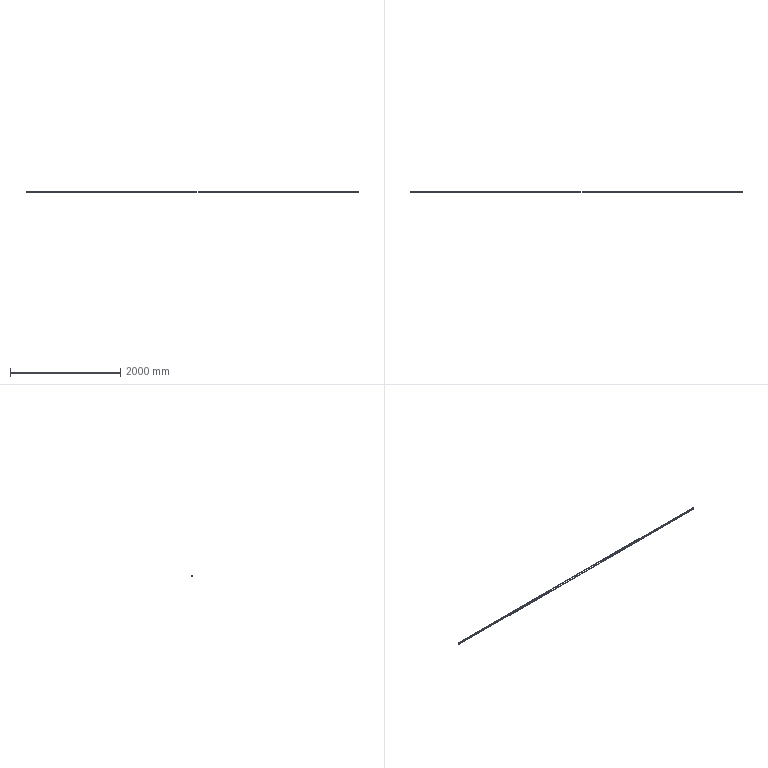Part | STEP file | ASND-0110-Q2 | 1 solid | 12 faces | box 6033 x 32.8 x 10 mm | volume 266115 mm3 | cylinder 6 | plane 6 | commonest cylinder face diameters 28.4 x3 32.8 x3
STEP:
#1=CARTESIAN_POINT('',(0.,0.,0.));
#2=DIRECTION('',(0.,0.,1.));
#3=DIRECTION('',(1.,0.,0.));
#4=AXIS2_PLACEMENT_3D('',#1,#2,#3);
#5=CARTESIAN_POINT('',(6000.,14.2,-140.));
#6=VERTEX_POINT('',#5);
#7=CARTESIAN_POINT('',(6000.,14.2,-130.));
#8=VERTEX_POINT('',#7);
#9=CARTESIAN_POINT('',(6000.,14.2,-140.));
#10=DIRECTION('',(0.,0.,1.));
#11=VECTOR('',#10,1.);
#12=LINE('',#9,#11);
#13=CARTESIAN_POINT('',(6000.,0.,-130.));
#14=DIRECTION('',(0.,0.,1.));
#15=DIRECTION('',(1.,0.,0.));
#16=AXIS2_PLACEMENT_3D('',#13,#14,#15);
#17=CYLINDRICAL_SURFACE('',#16,14.2);
#18=CARTESIAN_POINT('',(1.571,-10.));
#19=DIRECTION('',(0.,1.));
#20=VECTOR('',#19,1.);
#21=LINE('',#18,#20);
#22=(GEOMETRIC_REPRESENTATION_CONTEXT(2)PARAMETRIC_REPRESENTATION_CONTEXT()REPRESENTATION_CONTEXT('',''));
#23=DEFINITIONAL_REPRESENTATION('',(#21),#22);
#24=PCURVE('',#17,#23);
#25=CARTESIAN_POINT('',(0.,14.2,-130.));
#26=DIRECTION('',(0.,-1.,0.));
#27=DIRECTION('',(0.7071,0.,0.7071));
#28=AXIS2_PLACEMENT_3D('',#25,#26,#27);
#29=PLANE('',#28);
#30=CARTESIAN_POINT('',(4235.57,-4249.712));
#31=DIRECTION('',(0.7071,0.7071));
#32=VECTOR('',#31,1.);
#33=LINE('',#30,#32);
#34=(GEOMETRIC_REPRESENTATION_CONTEXT(2)PARAMETRIC_REPRESENTATION_CONTEXT()REPRESENTATION_CONTEXT('',''));
#35=DEFINITIONAL_REPRESENTATION('',(#33),#34);
#36=PCURVE('',#29,#35);
#37=SURFACE_CURVE('',#12,(#24,#36),.PCURVE_S1.);
#38=EDGE_CURVE('',#6,#8,#37,.T.);
#39=ORIENTED_EDGE('',*,*,#38,.T.);
#40=CARTESIAN_POINT('',(6014.2,0.,-130.));
#41=VERTEX_POINT('',#40);
#42=CARTESIAN_POINT('',(6000.,0.,-130.));
#43=DIRECTION('',(0.,0.,-1.));
#44=DIRECTION('',(1.,0.,0.));
#45=AXIS2_PLACEMENT_3D('',#42,#43,#44);
#46=CIRCLE('',#45,14.2);
#47=CARTESIAN_POINT('',(6.283,0.));
#48=DIRECTION('',(-1.,0.));
#49=VECTOR('',#48,1.);
#50=LINE('',#47,#49);
#51=(GEOMETRIC_REPRESENTATION_CONTEXT(2)PARAMETRIC_REPRESENTATION_CONTEXT()REPRESENTATION_CONTEXT('',''));
#52=DEFINITIONAL_REPRESENTATION('',(#50),#51);
#53=PCURVE('',#17,#52);
#54=CARTESIAN_POINT('',(0.,0.,-130.));
#55=DIRECTION('',(0.,0.,1.));
#56=DIRECTION('',(0.7071,0.7071,0.));
#57=AXIS2_PLACEMENT_3D('',#54,#55,#56);
#58=PLANE('',#57);
#59=CARTESIAN_POINT('',(4252.682,-4252.682));
#60=CARTESIAN_POINT('',(4235.29,-4270.073));
#61=CARTESIAN_POINT('',(4228.925,-4246.316));
#62=CARTESIAN_POINT('',(4222.559,-4222.559));
#63=CARTESIAN_POINT('',(4246.316,-4228.925));
#64=CARTESIAN_POINT('',(4270.073,-4235.29));
#65=CARTESIAN_POINT('',(4252.682,-4252.682));
#66=(BOUNDED_CURVE()B_SPLINE_CURVE(2,(#59,#60,#61,#62,#63,#64,#65),.UNSPECIFIED.,.T.,.F.)B_SPLINE_CURVE_WITH_KNOTS((1,2,2,2,2,1),(-2.094,0.,2.094,4.189,6.283,8.378),.UNSPECIFIED.)CURVE()GEOMETRIC_REPRESENTATION_ITEM()RATIONAL_B_SPLINE_CURVE((1.,0.5,1.,0.5,1.,0.5,1.))REPRESENTATION_ITEM(''));
#67=(GEOMETRIC_REPRESENTATION_CONTEXT(2)PARAMETRIC_REPRESENTATION_CONTEXT()REPRESENTATION_CONTEXT('',''));
#68=DEFINITIONAL_REPRESENTATION('',(#66),#67);
#69=PCURVE('',#58,#68);
#70=SURFACE_CURVE('',#46,(#53,#69),.PCURVE_S1.);
#71=EDGE_CURVE('',#8,#41,#70,.T.);
#72=ORIENTED_EDGE('',*,*,#71,.T.);
#73=CARTESIAN_POINT('',(6014.2,0.,-140.));
#74=VERTEX_POINT('',#73);
#75=CARTESIAN_POINT('',(6014.2,0.,-130.));
#76=DIRECTION('',(0.,0.,1.));
#77=VECTOR('',#76,1.);
#78=LINE('',#75,#77);
#79=CARTESIAN_POINT('',(0.,0.));
#80=DIRECTION('',(0.,1.));
#81=VECTOR('',#80,1.);
#82=LINE('',#79,#81);
#83=(GEOMETRIC_REPRESENTATION_CONTEXT(2)PARAMETRIC_REPRESENTATION_CONTEXT()REPRESENTATION_CONTEXT('',''));
#84=DEFINITIONAL_REPRESENTATION('',(#82),#83);
#85=PCURVE('',#17,#84);
#86=CARTESIAN_POINT('',(6000.,0.,-130.));
#87=DIRECTION('',(0.,0.,1.));
#88=DIRECTION('',(1.,0.,0.));
#89=AXIS2_PLACEMENT_3D('',#86,#87,#88);
#90=CYLINDRICAL_SURFACE('',#89,14.2);
#91=CARTESIAN_POINT('',(6.283,0.));
#92=DIRECTION('',(0.,1.));
#93=VECTOR('',#92,1.);
#94=LINE('',#91,#93);
#95=(GEOMETRIC_REPRESENTATION_CONTEXT(2)PARAMETRIC_REPRESENTATION_CONTEXT()REPRESENTATION_CONTEXT('',''));
#96=DEFINITIONAL_REPRESENTATION('',(#94),#95);
#97=PCURVE('',#90,#96);
#98=SURFACE_CURVE('',#78,(#85,#97),.PCURVE_S1.);
#99=EDGE_CURVE('',#74,#41,#98,.T.);
#100=ORIENTED_EDGE('',*,*,#99,.F.);
#101=CARTESIAN_POINT('',(6000.,0.,-140.));
#102=DIRECTION('',(0.,0.,1.));
#103=DIRECTION('',(1.,0.,0.));
#104=AXIS2_PLACEMENT_3D('',#101,#102,#103);
#105=CIRCLE('',#104,14.2);
#106=CARTESIAN_POINT('',(0.,-10.));
#107=DIRECTION('',(1.,0.));
#108=VECTOR('',#107,1.);
#109=LINE('',#106,#108);
#110=(GEOMETRIC_REPRESENTATION_CONTEXT(2)PARAMETRIC_REPRESENTATION_CONTEXT()REPRESENTATION_CONTEXT('',''));
#111=DEFINITIONAL_REPRESENTATION('',(#109),#110);
#112=PCURVE('',#17,#111);
#113=CARTESIAN_POINT('',(0.,0.,-140.));
#114=DIRECTION('',(0.,0.,1.));
#115=DIRECTION('',(0.7071,0.7071,0.));
#116=AXIS2_PLACEMENT_3D('',#113,#114,#115);
#117=PLANE('',#116);
#118=CARTESIAN_POINT('',(4242.641,-4242.641));
#119=DIRECTION('',(0.7071,-0.7071));
#120=AXIS2_PLACEMENT_2D('',#118,#119);
#121=CIRCLE('',#120,14.2);
#122=(GEOMETRIC_REPRESENTATION_CONTEXT(2)PARAMETRIC_REPRESENTATION_CONTEXT()REPRESENTATION_CONTEXT('',''));
#123=DEFINITIONAL_REPRESENTATION('',(#121),#122);
#124=PCURVE('',#117,#123);
#125=SURFACE_CURVE('',#105,(#112,#124),.PCURVE_S1.);
#126=EDGE_CURVE('',#74,#6,#125,.T.);
#127=ORIENTED_EDGE('',*,*,#126,.T.);
#128=EDGE_LOOP('',(#39,#72,#100,#127));
#129=FACE_BOUND('',#128,.F.);
#130=ADVANCED_FACE('',(#129),#17,.F.);
#131=CARTESIAN_POINT('',(6000.,-16.4,-140.));
#132=VERTEX_POINT('',#131);
#133=CARTESIAN_POINT('',(6016.4,0.,-140.));
#134=VERTEX_POINT('',#133);
#135=CARTESIAN_POINT('',(6000.,0.,-140.));
#136=DIRECTION('',(0.,0.,1.));
#137=DIRECTION('',(1.,0.,0.));
#138=AXIS2_PLACEMENT_3D('',#135,#136,#137);
#139=CIRCLE('',#138,16.4);
#140=CARTESIAN_POINT('',(6000.,0.,-130.));
#141=DIRECTION('',(0.,0.,1.));
#142=DIRECTION('',(1.,0.,0.));
#143=AXIS2_PLACEMENT_3D('',#140,#141,#142);
#144=CYLINDRICAL_SURFACE('',#143,16.4);
#145=CARTESIAN_POINT('',(0.,-10.));
#146=DIRECTION('',(1.,0.));
#147=VECTOR('',#146,1.);
#148=LINE('',#145,#147);
#149=(GEOMETRIC_REPRESENTATION_CONTEXT(2)PARAMETRIC_REPRESENTATION_CONTEXT()REPRESENTATION_CONTEXT('',''));
#150=DEFINITIONAL_REPRESENTATION('',(#148),#149);
#151=PCURVE('',#144,#150);
#152=CARTESIAN_POINT('',(4242.641,-4242.641));
#153=DIRECTION('',(0.7071,-0.7071));
#154=AXIS2_PLACEMENT_2D('',#152,#153);
#155=CIRCLE('',#154,16.4);
#156=(GEOMETRIC_REPRESENTATION_CONTEXT(2)PARAMETRIC_REPRESENTATION_CONTEXT()REPRESENTATION_CONTEXT('',''));
#157=DEFINITIONAL_REPRESENTATION('',(#155),#156);
#158=PCURVE('',#117,#157);
#159=SURFACE_CURVE('',#139,(#151,#158),.PCURVE_S1.);
#160=EDGE_CURVE('',#132,#134,#159,.T.);
#161=ORIENTED_EDGE('',*,*,#160,.T.);
#162=CARTESIAN_POINT('',(6016.4,0.,-130.));
#163=VERTEX_POINT('',#162);
#164=CARTESIAN_POINT('',(6016.4,0.,-130.));
#165=DIRECTION('',(0.,0.,1.));
#166=VECTOR('',#165,1.);
#167=LINE('',#164,#166);
#168=CARTESIAN_POINT('',(6.283,0.));
#169=DIRECTION('',(0.,1.));
#170=VECTOR('',#169,1.);
#171=LINE('',#168,#170);
#172=(GEOMETRIC_REPRESENTATION_CONTEXT(2)PARAMETRIC_REPRESENTATION_CONTEXT()REPRESENTATION_CONTEXT('',''));
#173=DEFINITIONAL_REPRESENTATION('',(#171),#172);
#174=PCURVE('',#144,#173);
#175=CARTESIAN_POINT('',(6000.,0.,-130.));
#176=DIRECTION('',(0.,0.,1.));
#177=DIRECTION('',(1.,0.,0.));
#178=AXIS2_PLACEMENT_3D('',#175,#176,#177);
#179=CYLINDRICAL_SURFACE('',#178,16.4);
#180=CARTESIAN_POINT('',(0.,0.));
#181=DIRECTION('',(0.,1.));
#182=VECTOR('',#181,1.);
#183=LINE('',#180,#182);
#184=(GEOMETRIC_REPRESENTATION_CONTEXT(2)PARAMETRIC_REPRESENTATION_CONTEXT()REPRESENTATION_CONTEXT('',''));
#185=DEFINITIONAL_REPRESENTATION('',(#183),#184);
#186=PCURVE('',#179,#185);
#187=SURFACE_CURVE('',#167,(#174,#186),.PCURVE_S1.);
#188=EDGE_CURVE('',#134,#163,#187,.T.);
#189=ORIENTED_EDGE('',*,*,#188,.T.);
#190=CARTESIAN_POINT('',(6000.,-16.4,-130.));
#191=VERTEX_POINT('',#190);
#192=CARTESIAN_POINT('',(6000.,0.,-130.));
#193=DIRECTION('',(0.,0.,1.));
#194=DIRECTION('',(1.,0.,0.));
#195=AXIS2_PLACEMENT_3D('',#192,#193,#194);
#196=CIRCLE('',#195,16.4);
#197=CARTESIAN_POINT('',(0.,0.));
#198=DIRECTION('',(1.,0.));
#199=VECTOR('',#198,1.);
#200=LINE('',#197,#199);
#201=(GEOMETRIC_REPRESENTATION_CONTEXT(2)PARAMETRIC_REPRESENTATION_CONTEXT()REPRESENTATION_CONTEXT('',''));
#202=DEFINITIONAL_REPRESENTATION('',(#200),#201);
#203=PCURVE('',#144,#202);
#204=CARTESIAN_POINT('',(4242.641,-4242.641));
#205=DIRECTION('',(0.7071,-0.7071));
#206=AXIS2_PLACEMENT_2D('',#204,#205);
#207=CIRCLE('',#206,16.4);
#208=(GEOMETRIC_REPRESENTATION_CONTEXT(2)PARAMETRIC_REPRESENTATION_CONTEXT()REPRESENTATION_CONTEXT('',''));
#209=DEFINITIONAL_REPRESENTATION('',(#207),#208);
#210=PCURVE('',#58,#209);
#211=SURFACE_CURVE('',#196,(#203,#210),.PCURVE_S1.);
#212=EDGE_CURVE('',#191,#163,#211,.T.);
#213=ORIENTED_EDGE('',*,*,#212,.F.);
#214=CARTESIAN_POINT('',(6000.,-16.4,-140.));
#215=DIRECTION('',(0.,0.,-1.));
#216=VECTOR('',#215,1.);
#217=LINE('',#214,#216);
#218=CARTESIAN_POINT('',(4.712,-10.));
#219=DIRECTION('',(0.,-1.));
#220=VECTOR('',#219,1.);
#221=LINE('',#218,#220);
#222=(GEOMETRIC_REPRESENTATION_CONTEXT(2)PARAMETRIC_REPRESENTATION_CONTEXT()REPRESENTATION_CONTEXT('',''));
#223=DEFINITIONAL_REPRESENTATION('',(#221),#222);
#224=PCURVE('',#144,#223);
#225=CARTESIAN_POINT('',(0.,-16.4,-130.));
#226=DIRECTION('',(0.,-1.,0.));
#227=DIRECTION('',(0.7071,0.,0.7071));
#228=AXIS2_PLACEMENT_3D('',#225,#226,#227);
#229=PLANE('',#228);
#230=CARTESIAN_POINT('',(4235.57,-4249.712));
#231=DIRECTION('',(-0.7071,-0.7071));
#232=VECTOR('',#231,1.);
#233=LINE('',#230,#232);
#234=(GEOMETRIC_REPRESENTATION_CONTEXT(2)PARAMETRIC_REPRESENTATION_CONTEXT()REPRESENTATION_CONTEXT('',''));
#235=DEFINITIONAL_REPRESENTATION('',(#233),#234);
#236=PCURVE('',#229,#235);
#237=SURFACE_CURVE('',#217,(#224,#236),.PCURVE_S1.);
#238=EDGE_CURVE('',#191,#132,#237,.T.);
#239=ORIENTED_EDGE('',*,*,#238,.T.);
#240=EDGE_LOOP('',(#161,#189,#213,#239));
#241=FACE_BOUND('',#240,.T.);
#242=ADVANCED_FACE('',(#241),#144,.T.);
#243=CARTESIAN_POINT('',(0.,16.4,-130.));
#244=VERTEX_POINT('',#243);
#245=CARTESIAN_POINT('',(0.,-16.4,-130.));
#246=VERTEX_POINT('',#245);
#247=CARTESIAN_POINT('',(0.,0.,-130.));
#248=DIRECTION('',(0.,0.,1.));
#249=DIRECTION('',(1.,0.,0.));
#250=AXIS2_PLACEMENT_3D('',#247,#248,#249);
#251=CIRCLE('',#250,16.4);
#252=CARTESIAN_POINT('',(0.,0.,-130.));
#253=DIRECTION('',(0.,0.,1.));
#254=DIRECTION('',(1.,0.,0.));
#255=AXIS2_PLACEMENT_3D('',#252,#253,#254);
#256=CYLINDRICAL_SURFACE('',#255,16.4);
#257=CARTESIAN_POINT('',(0.,0.));
#258=DIRECTION('',(1.,0.));
#259=VECTOR('',#258,1.);
#260=LINE('',#257,#259);
#261=(GEOMETRIC_REPRESENTATION_CONTEXT(2)PARAMETRIC_REPRESENTATION_CONTEXT()REPRESENTATION_CONTEXT('',''));
#262=DEFINITIONAL_REPRESENTATION('',(#260),#261);
#263=PCURVE('',#256,#262);
#264=CARTESIAN_POINT('',(0.,0.));
#265=DIRECTION('',(0.7071,-0.7071));
#266=AXIS2_PLACEMENT_2D('',#264,#265);
#267=CIRCLE('',#266,16.4);
#268=(GEOMETRIC_REPRESENTATION_CONTEXT(2)PARAMETRIC_REPRESENTATION_CONTEXT()REPRESENTATION_CONTEXT('',''));
#269=DEFINITIONAL_REPRESENTATION('',(#267),#268);
#270=PCURVE('',#58,#269);
#271=SURFACE_CURVE('',#251,(#263,#270),.PCURVE_S1.);
#272=EDGE_CURVE('',#244,#246,#271,.T.);
#273=ORIENTED_EDGE('',*,*,#272,.F.);
#274=CARTESIAN_POINT('',(0.,16.4,-140.));
#275=VERTEX_POINT('',#274);
#276=CARTESIAN_POINT('',(0.,16.4,-140.));
#277=DIRECTION('',(0.,0.,1.));
#278=VECTOR('',#277,1.);
#279=LINE('',#276,#278);
#280=CARTESIAN_POINT('',(1.571,-10.));
#281=DIRECTION('',(0.,1.));
#282=VECTOR('',#281,1.);
#283=LINE('',#280,#282);
#284=(GEOMETRIC_REPRESENTATION_CONTEXT(2)PARAMETRIC_REPRESENTATION_CONTEXT()REPRESENTATION_CONTEXT('',''));
#285=DEFINITIONAL_REPRESENTATION('',(#283),#284);
#286=PCURVE('',#256,#285);
#287=CARTESIAN_POINT('',(3000.,16.4,-130.));
#288=DIRECTION('',(0.,1.,0.));
#289=DIRECTION('',(0.7071,0.,0.7071));
#290=AXIS2_PLACEMENT_3D('',#287,#288,#289);
#291=PLANE('',#290);
#292=CARTESIAN_POINT('',(-2128.391,-2114.249));
#293=DIRECTION('',(0.7071,-0.7071));
#294=VECTOR('',#293,1.);
#295=LINE('',#292,#294);
#296=(GEOMETRIC_REPRESENTATION_CONTEXT(2)PARAMETRIC_REPRESENTATION_CONTEXT()REPRESENTATION_CONTEXT('',''));
#297=DEFINITIONAL_REPRESENTATION('',(#295),#296);
#298=PCURVE('',#291,#297);
#299=SURFACE_CURVE('',#279,(#286,#298),.PCURVE_S1.);
#300=EDGE_CURVE('',#275,#244,#299,.T.);
#301=ORIENTED_EDGE('',*,*,#300,.F.);
#302=CARTESIAN_POINT('',(0.,-16.4,-140.));
#303=VERTEX_POINT('',#302);
#304=CARTESIAN_POINT('',(0.,0.,-140.));
#305=DIRECTION('',(0.,0.,1.));
#306=DIRECTION('',(1.,0.,0.));
#307=AXIS2_PLACEMENT_3D('',#304,#305,#306);
#308=CIRCLE('',#307,16.4);
#309=CARTESIAN_POINT('',(0.,-10.));
#310=DIRECTION('',(1.,0.));
#311=VECTOR('',#310,1.);
#312=LINE('',#309,#311);
#313=(GEOMETRIC_REPRESENTATION_CONTEXT(2)PARAMETRIC_REPRESENTATION_CONTEXT()REPRESENTATION_CONTEXT('',''));
#314=DEFINITIONAL_REPRESENTATION('',(#312),#313);
#315=PCURVE('',#256,#314);
#316=CARTESIAN_POINT('',(0.,0.));
#317=DIRECTION('',(0.7071,-0.7071));
#318=AXIS2_PLACEMENT_2D('',#316,#317);
#319=CIRCLE('',#318,16.4);
#320=(GEOMETRIC_REPRESENTATION_CONTEXT(2)PARAMETRIC_REPRESENTATION_CONTEXT()REPRESENTATION_CONTEXT('',''));
#321=DEFINITIONAL_REPRESENTATION('',(#319),#320);
#322=PCURVE('',#117,#321);
#323=SURFACE_CURVE('',#308,(#315,#322),.PCURVE_S1.);
#324=EDGE_CURVE('',#275,#303,#323,.T.);
#325=ORIENTED_EDGE('',*,*,#324,.T.);
#326=CARTESIAN_POINT('',(0.,-16.4,-130.));
#327=DIRECTION('',(0.,0.,-1.));
#328=VECTOR('',#327,1.);
#329=LINE('',#326,#328);
#330=CARTESIAN_POINT('',(4.712,0.));
#331=DIRECTION('',(0.,-1.));
#332=VECTOR('',#331,1.);
#333=LINE('',#330,#332);
#334=(GEOMETRIC_REPRESENTATION_CONTEXT(2)PARAMETRIC_REPRESENTATION_CONTEXT()REPRESENTATION_CONTEXT('',''));
#335=DEFINITIONAL_REPRESENTATION('',(#333),#334);
#336=PCURVE('',#256,#335);
#337=CARTESIAN_POINT('',(0.,0.));
#338=DIRECTION('',(-0.7071,-0.7071));
#339=VECTOR('',#338,1.);
#340=LINE('',#337,#339);
#341=(GEOMETRIC_REPRESENTATION_CONTEXT(2)PARAMETRIC_REPRESENTATION_CONTEXT()REPRESENTATION_CONTEXT('',''));
#342=DEFINITIONAL_REPRESENTATION('',(#340),#341);
#343=PCURVE('',#229,#342);
#344=SURFACE_CURVE('',#329,(#336,#343),.PCURVE_S1.);
#345=EDGE_CURVE('',#246,#303,#344,.T.);
#346=ORIENTED_EDGE('',*,*,#345,.F.);
#347=EDGE_LOOP('',(#273,#301,#325,#346));
#348=FACE_BOUND('',#347,.T.);
#349=ADVANCED_FACE('',(#348),#256,.T.);
#350=CARTESIAN_POINT('',(0.,-16.4,-130.));
#351=DIRECTION('',(1.,0.,0.));
#352=VECTOR('',#351,1.);
#353=LINE('',#350,#352);
#354=CARTESIAN_POINT('',(0.,0.));
#355=DIRECTION('',(0.7071,-0.7071));
#356=VECTOR('',#355,1.);
#357=LINE('',#354,#356);
#358=(GEOMETRIC_REPRESENTATION_CONTEXT(2)PARAMETRIC_REPRESENTATION_CONTEXT()REPRESENTATION_CONTEXT('',''));
#359=DEFINITIONAL_REPRESENTATION('',(#357),#358);
#360=PCURVE('',#229,#359);
#361=CARTESIAN_POINT('',(-11.597,-11.597));
#362=DIRECTION('',(0.7071,-0.7071));
#363=VECTOR('',#362,1.);
#364=LINE('',#361,#363);
#365=(GEOMETRIC_REPRESENTATION_CONTEXT(2)PARAMETRIC_REPRESENTATION_CONTEXT()REPRESENTATION_CONTEXT('',''));
#366=DEFINITIONAL_REPRESENTATION('',(#364),#365);
#367=PCURVE('',#58,#366);
#368=SURFACE_CURVE('',#353,(#360,#367),.PCURVE_S1.);
#369=EDGE_CURVE('',#246,#191,#368,.T.);
#370=ORIENTED_EDGE('',*,*,#369,.F.);
#371=ORIENTED_EDGE('',*,*,#345,.T.);
#372=CARTESIAN_POINT('',(0.,-16.4,-140.));
#373=DIRECTION('',(1.,0.,0.));
#374=VECTOR('',#373,1.);
#375=LINE('',#372,#374);
#376=CARTESIAN_POINT('',(-7.071,-7.071));
#377=DIRECTION('',(0.7071,-0.7071));
#378=VECTOR('',#377,1.);
#379=LINE('',#376,#378);
#380=(GEOMETRIC_REPRESENTATION_CONTEXT(2)PARAMETRIC_REPRESENTATION_CONTEXT()REPRESENTATION_CONTEXT('',''));
#381=DEFINITIONAL_REPRESENTATION('',(#379),#380);
#382=PCURVE('',#229,#381);
#383=CARTESIAN_POINT('',(-11.597,-11.597));
#384=DIRECTION('',(0.7071,-0.7071));
#385=VECTOR('',#384,1.);
#386=LINE('',#383,#385);
#387=(GEOMETRIC_REPRESENTATION_CONTEXT(2)PARAMETRIC_REPRESENTATION_CONTEXT()REPRESENTATION_CONTEXT('',''));
#388=DEFINITIONAL_REPRESENTATION('',(#386),#387);
#389=PCURVE('',#117,#388);
#390=SURFACE_CURVE('',#375,(#382,#389),.PCURVE_S1.);
#391=EDGE_CURVE('',#303,#132,#390,.T.);
#392=ORIENTED_EDGE('',*,*,#391,.T.);
#393=ORIENTED_EDGE('',*,*,#238,.F.);
#394=EDGE_LOOP('',(#370,#371,#392,#393));
#395=FACE_BOUND('',#394,.T.);
#396=ADVANCED_FACE('',(#395),#229,.T.);
#397=ORIENTED_EDGE('',*,*,#188,.F.);
#398=CARTESIAN_POINT('',(6000.,16.4,-140.));
#399=VERTEX_POINT('',#398);
#400=CARTESIAN_POINT('',(6000.,0.,-140.));
#401=DIRECTION('',(0.,0.,1.));
#402=DIRECTION('',(1.,0.,0.));
#403=AXIS2_PLACEMENT_3D('',#400,#401,#402);
#404=CIRCLE('',#403,16.4);
#405=CARTESIAN_POINT('',(0.,-10.));
#406=DIRECTION('',(1.,0.));
#407=VECTOR('',#406,1.);
#408=LINE('',#405,#407);
#409=(GEOMETRIC_REPRESENTATION_CONTEXT(2)PARAMETRIC_REPRESENTATION_CONTEXT()REPRESENTATION_CONTEXT('',''));
#410=DEFINITIONAL_REPRESENTATION('',(#408),#409);
#411=PCURVE('',#179,#410);
#412=CARTESIAN_POINT('',(4242.641,-4242.641));
#413=DIRECTION('',(0.7071,-0.7071));
#414=AXIS2_PLACEMENT_2D('',#412,#413);
#415=CIRCLE('',#414,16.4);
#416=(GEOMETRIC_REPRESENTATION_CONTEXT(2)PARAMETRIC_REPRESENTATION_CONTEXT()REPRESENTATION_CONTEXT('',''));
#417=DEFINITIONAL_REPRESENTATION('',(#415),#416);
#418=PCURVE('',#117,#417);
#419=SURFACE_CURVE('',#404,(#411,#418),.PCURVE_S1.);
#420=EDGE_CURVE('',#134,#399,#419,.T.);
#421=ORIENTED_EDGE('',*,*,#420,.T.);
#422=CARTESIAN_POINT('',(6000.,16.4,-130.));
#423=VERTEX_POINT('',#422);
#424=CARTESIAN_POINT('',(6000.,16.4,-140.));
#425=DIRECTION('',(0.,0.,-1.));
#426=VECTOR('',#425,1.);
#427=LINE('',#424,#426);
#428=CARTESIAN_POINT('',(1.571,-10.));
#429=DIRECTION('',(0.,-1.));
#430=VECTOR('',#429,1.);
#431=LINE('',#428,#430);
#432=(GEOMETRIC_REPRESENTATION_CONTEXT(2)PARAMETRIC_REPRESENTATION_CONTEXT()REPRESENTATION_CONTEXT('',''));
#433=DEFINITIONAL_REPRESENTATION('',(#431),#432);
#434=PCURVE('',#179,#433);
#435=CARTESIAN_POINT('',(2114.249,2128.391));
#436=DIRECTION('',(-0.7071,0.7071));
#437=VECTOR('',#436,1.);
#438=LINE('',#435,#437);
#439=(GEOMETRIC_REPRESENTATION_CONTEXT(2)PARAMETRIC_REPRESENTATION_CONTEXT()REPRESENTATION_CONTEXT('',''));
#440=DEFINITIONAL_REPRESENTATION('',(#438),#439);
#441=PCURVE('',#291,#440);
#442=SURFACE_CURVE('',#427,(#434,#441),.PCURVE_S1.);
#443=EDGE_CURVE('',#423,#399,#442,.T.);
#444=ORIENTED_EDGE('',*,*,#443,.F.);
#445=CARTESIAN_POINT('',(6000.,0.,-130.));
#446=DIRECTION('',(0.,0.,1.));
#447=DIRECTION('',(1.,0.,0.));
#448=AXIS2_PLACEMENT_3D('',#445,#446,#447);
#449=CIRCLE('',#448,16.4);
#450=CARTESIAN_POINT('',(0.,0.));
#451=DIRECTION('',(1.,0.));
#452=VECTOR('',#451,1.);
#453=LINE('',#450,#452);
#454=(GEOMETRIC_REPRESENTATION_CONTEXT(2)PARAMETRIC_REPRESENTATION_CONTEXT()REPRESENTATION_CONTEXT('',''));
#455=DEFINITIONAL_REPRESENTATION('',(#453),#454);
#456=PCURVE('',#179,#455);
#457=CARTESIAN_POINT('',(4242.641,-4242.641));
#458=DIRECTION('',(0.7071,-0.7071));
#459=AXIS2_PLACEMENT_2D('',#457,#458);
#460=CIRCLE('',#459,16.4);
#461=(GEOMETRIC_REPRESENTATION_CONTEXT(2)PARAMETRIC_REPRESENTATION_CONTEXT()REPRESENTATION_CONTEXT('',''));
#462=DEFINITIONAL_REPRESENTATION('',(#460),#461);
#463=PCURVE('',#58,#462);
#464=SURFACE_CURVE('',#449,(#456,#463),.PCURVE_S1.);
#465=EDGE_CURVE('',#163,#423,#464,.T.);
#466=ORIENTED_EDGE('',*,*,#465,.F.);
#467=EDGE_LOOP('',(#397,#421,#444,#466));
#468=FACE_BOUND('',#467,.T.);
#469=ADVANCED_FACE('',(#468),#179,.T.);
#470=CARTESIAN_POINT('',(0.,16.4,-130.));
#471=DIRECTION('',(-1.,0.,0.));
#472=VECTOR('',#471,1.);
#473=LINE('',#470,#472);
#474=CARTESIAN_POINT('',(-2121.32,-2121.32));
#475=DIRECTION('',(-0.7071,-0.7071));
#476=VECTOR('',#475,1.);
#477=LINE('',#474,#476);
#478=(GEOMETRIC_REPRESENTATION_CONTEXT(2)PARAMETRIC_REPRESENTATION_CONTEXT()REPRESENTATION_CONTEXT('',''));
#479=DEFINITIONAL_REPRESENTATION('',(#477),#478);
#480=PCURVE('',#291,#479);
#481=CARTESIAN_POINT('',(11.597,11.597));
#482=DIRECTION('',(-0.7071,0.7071));
#483=VECTOR('',#482,1.);
#484=LINE('',#481,#483);
#485=(GEOMETRIC_REPRESENTATION_CONTEXT(2)PARAMETRIC_REPRESENTATION_CONTEXT()REPRESENTATION_CONTEXT('',''));
#486=DEFINITIONAL_REPRESENTATION('',(#484),#485);
#487=PCURVE('',#58,#486);
#488=SURFACE_CURVE('',#473,(#480,#487),.PCURVE_S1.);
#489=EDGE_CURVE('',#423,#244,#488,.T.);
#490=ORIENTED_EDGE('',*,*,#489,.F.);
#491=ORIENTED_EDGE('',*,*,#443,.T.);
#492=CARTESIAN_POINT('',(0.,16.4,-140.));
#493=DIRECTION('',(-1.,0.,0.));
#494=VECTOR('',#493,1.);
#495=LINE('',#492,#494);
#496=CARTESIAN_POINT('',(-2128.391,-2114.249));
#497=DIRECTION('',(-0.7071,-0.7071));
#498=VECTOR('',#497,1.);
#499=LINE('',#496,#498);
#500=(GEOMETRIC_REPRESENTATION_CONTEXT(2)PARAMETRIC_REPRESENTATION_CONTEXT()REPRESENTATION_CONTEXT('',''));
#501=DEFINITIONAL_REPRESENTATION('',(#499),#500);
#502=PCURVE('',#291,#501);
#503=CARTESIAN_POINT('',(11.597,11.597));
#504=DIRECTION('',(-0.7071,0.7071));
#505=VECTOR('',#504,1.);
#506=LINE('',#503,#505);
#507=(GEOMETRIC_REPRESENTATION_CONTEXT(2)PARAMETRIC_REPRESENTATION_CONTEXT()REPRESENTATION_CONTEXT('',''));
#508=DEFINITIONAL_REPRESENTATION('',(#506),#507);
#509=PCURVE('',#117,#508);
#510=SURFACE_CURVE('',#495,(#502,#509),.PCURVE_S1.);
#511=EDGE_CURVE('',#399,#275,#510,.T.);
#512=ORIENTED_EDGE('',*,*,#511,.T.);
#513=ORIENTED_EDGE('',*,*,#300,.T.);
#514=EDGE_LOOP('',(#490,#491,#512,#513));
#515=FACE_BOUND('',#514,.T.);
#516=ADVANCED_FACE('',(#515),#291,.T.);
#517=CARTESIAN_POINT('',(0.,14.2,-130.));
#518=VERTEX_POINT('',#517);
#519=CARTESIAN_POINT('',(0.,14.2,-130.));
#520=DIRECTION('',(1.,0.,0.));
#521=VECTOR('',#520,1.);
#522=LINE('',#519,#521);
#523=CARTESIAN_POINT('',(0.,0.));
#524=DIRECTION('',(0.7071,-0.7071));
#525=VECTOR('',#524,1.);
#526=LINE('',#523,#525);
#527=(GEOMETRIC_REPRESENTATION_CONTEXT(2)PARAMETRIC_REPRESENTATION_CONTEXT()REPRESENTATION_CONTEXT('',''));
#528=DEFINITIONAL_REPRESENTATION('',(#526),#527);
#529=PCURVE('',#29,#528);
#530=CARTESIAN_POINT('',(10.041,10.041));
#531=DIRECTION('',(0.7071,-0.7071));
#532=VECTOR('',#531,1.);
#533=LINE('',#530,#532);
#534=(GEOMETRIC_REPRESENTATION_CONTEXT(2)PARAMETRIC_REPRESENTATION_CONTEXT()REPRESENTATION_CONTEXT('',''));
#535=DEFINITIONAL_REPRESENTATION('',(#533),#534);
#536=PCURVE('',#58,#535);
#537=SURFACE_CURVE('',#522,(#529,#536),.PCURVE_S1.);
#538=EDGE_CURVE('',#518,#8,#537,.T.);
#539=ORIENTED_EDGE('',*,*,#538,.F.);
#540=CARTESIAN_POINT('',(0.,14.2,-140.));
#541=VERTEX_POINT('',#540);
#542=CARTESIAN_POINT('',(0.,14.2,-140.));
#543=DIRECTION('',(0.,0.,-1.));
#544=VECTOR('',#543,1.);
#545=LINE('',#542,#544);
#546=CARTESIAN_POINT('',(-7.071,-7.071));
#547=DIRECTION('',(-0.7071,-0.7071));
#548=VECTOR('',#547,1.);
#549=LINE('',#546,#548);
#550=(GEOMETRIC_REPRESENTATION_CONTEXT(2)PARAMETRIC_REPRESENTATION_CONTEXT()REPRESENTATION_CONTEXT('',''));
#551=DEFINITIONAL_REPRESENTATION('',(#549),#550);
#552=PCURVE('',#29,#551);
#553=CARTESIAN_POINT('',(0.,0.,-130.));
#554=DIRECTION('',(0.,0.,1.));
#555=DIRECTION('',(1.,0.,0.));
#556=AXIS2_PLACEMENT_3D('',#553,#554,#555);
#557=CYLINDRICAL_SURFACE('',#556,14.2);
#558=CARTESIAN_POINT('',(1.571,-10.));
#559=DIRECTION('',(0.,-1.));
#560=VECTOR('',#559,1.);
#561=LINE('',#558,#560);
#562=(GEOMETRIC_REPRESENTATION_CONTEXT(2)PARAMETRIC_REPRESENTATION_CONTEXT()REPRESENTATION_CONTEXT('',''));
#563=DEFINITIONAL_REPRESENTATION('',(#561),#562);
#564=PCURVE('',#557,#563);
#565=SURFACE_CURVE('',#545,(#552,#564),.PCURVE_S1.);
#566=EDGE_CURVE('',#518,#541,#565,.T.);
#567=ORIENTED_EDGE('',*,*,#566,.T.);
#568=CARTESIAN_POINT('',(0.,14.2,-140.));
#569=DIRECTION('',(1.,0.,0.));
#570=VECTOR('',#569,1.);
#571=LINE('',#568,#570);
#572=CARTESIAN_POINT('',(-7.071,-7.071));
#573=DIRECTION('',(0.7071,-0.7071));
#574=VECTOR('',#573,1.);
#575=LINE('',#572,#574);
#576=(GEOMETRIC_REPRESENTATION_CONTEXT(2)PARAMETRIC_REPRESENTATION_CONTEXT()REPRESENTATION_CONTEXT('',''));
#577=DEFINITIONAL_REPRESENTATION('',(#575),#576);
#578=PCURVE('',#29,#577);
#579=CARTESIAN_POINT('',(10.041,10.041));
#580=DIRECTION('',(0.7071,-0.7071));
#581=VECTOR('',#580,1.);
#582=LINE('',#579,#581);
#583=(GEOMETRIC_REPRESENTATION_CONTEXT(2)PARAMETRIC_REPRESENTATION_CONTEXT()REPRESENTATION_CONTEXT('',''));
#584=DEFINITIONAL_REPRESENTATION('',(#582),#583);
#585=PCURVE('',#117,#584);
#586=SURFACE_CURVE('',#571,(#578,#585),.PCURVE_S1.);
#587=EDGE_CURVE('',#541,#6,#586,.T.);
#588=ORIENTED_EDGE('',*,*,#587,.T.);
#589=ORIENTED_EDGE('',*,*,#38,.T.);
#590=EDGE_LOOP('',(#539,#567,#588,#589));
#591=FACE_BOUND('',#590,.T.);
#592=ADVANCED_FACE('',(#591),#29,.T.);
#593=ORIENTED_EDGE('',*,*,#324,.F.);
#594=ORIENTED_EDGE('',*,*,#511,.F.);
#595=ORIENTED_EDGE('',*,*,#420,.F.);
#596=ORIENTED_EDGE('',*,*,#160,.F.);
#597=ORIENTED_EDGE('',*,*,#391,.F.);
#598=EDGE_LOOP('',(#593,#594,#595,#596,#597));
#599=FACE_BOUND('',#598,.T.);
#600=ORIENTED_EDGE('',*,*,#587,.F.);
#601=CARTESIAN_POINT('',(0.,-14.2,-140.));
#602=VERTEX_POINT('',#601);
#603=CARTESIAN_POINT('',(0.,0.,-140.));
#604=DIRECTION('',(0.,0.,1.));
#605=DIRECTION('',(1.,0.,0.));
#606=AXIS2_PLACEMENT_3D('',#603,#604,#605);
#607=CIRCLE('',#606,14.2);
#608=CARTESIAN_POINT('',(0.,0.));
#609=DIRECTION('',(0.7071,-0.7071));
#610=AXIS2_PLACEMENT_2D('',#608,#609);
#611=CIRCLE('',#610,14.2);
#612=(GEOMETRIC_REPRESENTATION_CONTEXT(2)PARAMETRIC_REPRESENTATION_CONTEXT()REPRESENTATION_CONTEXT('',''));
#613=DEFINITIONAL_REPRESENTATION('',(#611),#612);
#614=PCURVE('',#117,#613);
#615=CARTESIAN_POINT('',(0.,-10.));
#616=DIRECTION('',(1.,0.));
#617=VECTOR('',#616,1.);
#618=LINE('',#615,#617);
#619=(GEOMETRIC_REPRESENTATION_CONTEXT(2)PARAMETRIC_REPRESENTATION_CONTEXT()REPRESENTATION_CONTEXT('',''));
#620=DEFINITIONAL_REPRESENTATION('',(#618),#619);
#621=PCURVE('',#557,#620);
#622=SURFACE_CURVE('',#607,(#614,#621),.PCURVE_S1.);
#623=EDGE_CURVE('',#541,#602,#622,.T.);
#624=ORIENTED_EDGE('',*,*,#623,.T.);
#625=CARTESIAN_POINT('',(6000.,-14.2,-140.));
#626=VERTEX_POINT('',#625);
#627=CARTESIAN_POINT('',(0.,-14.2,-140.));
#628=DIRECTION('',(-1.,0.,0.));
#629=VECTOR('',#628,1.);
#630=LINE('',#627,#629);
#631=CARTESIAN_POINT('',(-10.041,-10.041));
#632=DIRECTION('',(-0.7071,0.7071));
#633=VECTOR('',#632,1.);
#634=LINE('',#631,#633);
#635=(GEOMETRIC_REPRESENTATION_CONTEXT(2)PARAMETRIC_REPRESENTATION_CONTEXT()REPRESENTATION_CONTEXT('',''));
#636=DEFINITIONAL_REPRESENTATION('',(#634),#635);
#637=PCURVE('',#117,#636);
#638=CARTESIAN_POINT('',(3000.,-14.2,-130.));
#639=DIRECTION('',(0.,1.,0.));
#640=DIRECTION('',(0.7071,0.,0.7071));
#641=AXIS2_PLACEMENT_3D('',#638,#639,#640);
#642=PLANE('',#641);
#643=CARTESIAN_POINT('',(-2128.391,-2114.249));
#644=DIRECTION('',(-0.7071,-0.7071));
#645=VECTOR('',#644,1.);
#646=LINE('',#643,#645);
#647=(GEOMETRIC_REPRESENTATION_CONTEXT(2)PARAMETRIC_REPRESENTATION_CONTEXT()REPRESENTATION_CONTEXT('',''));
#648=DEFINITIONAL_REPRESENTATION('',(#646),#647);
#649=PCURVE('',#642,#648);
#650=SURFACE_CURVE('',#630,(#637,#649),.PCURVE_S1.);
#651=EDGE_CURVE('',#626,#602,#650,.T.);
#652=ORIENTED_EDGE('',*,*,#651,.F.);
#653=CARTESIAN_POINT('',(6000.,0.,-140.));
#654=DIRECTION('',(0.,0.,1.));
#655=DIRECTION('',(1.,0.,0.));
#656=AXIS2_PLACEMENT_3D('',#653,#654,#655);
#657=CIRCLE('',#656,14.2);
#658=CARTESIAN_POINT('',(4242.641,-4242.641));
#659=DIRECTION('',(0.7071,-0.7071));
#660=AXIS2_PLACEMENT_2D('',#658,#659);
#661=CIRCLE('',#660,14.2);
#662=(GEOMETRIC_REPRESENTATION_CONTEXT(2)PARAMETRIC_REPRESENTATION_CONTEXT()REPRESENTATION_CONTEXT('',''));
#663=DEFINITIONAL_REPRESENTATION('',(#661),#662);
#664=PCURVE('',#117,#663);
#665=CARTESIAN_POINT('',(0.,-10.));
#666=DIRECTION('',(1.,0.));
#667=VECTOR('',#666,1.);
#668=LINE('',#665,#667);
#669=(GEOMETRIC_REPRESENTATION_CONTEXT(2)PARAMETRIC_REPRESENTATION_CONTEXT()REPRESENTATION_CONTEXT('',''));
#670=DEFINITIONAL_REPRESENTATION('',(#668),#669);
#671=PCURVE('',#90,#670);
#672=SURFACE_CURVE('',#657,(#664,#671),.PCURVE_S1.);
#673=EDGE_CURVE('',#626,#74,#672,.T.);
#674=ORIENTED_EDGE('',*,*,#673,.T.);
#675=ORIENTED_EDGE('',*,*,#126,.T.);
#676=EDGE_LOOP('',(#600,#624,#652,#674,#675));
#677=FACE_BOUND('',#676,.T.);
#678=ADVANCED_FACE('',(#599,#677),#117,.F.);
#679=ORIENTED_EDGE('',*,*,#623,.T.);
#680=CARTESIAN_POINT('',(0.,-14.2,-130.));
#681=VERTEX_POINT('',#680);
#682=CARTESIAN_POINT('',(0.,-14.2,-140.));
#683=DIRECTION('',(0.,0.,1.));
#684=VECTOR('',#683,1.);
#685=LINE('',#682,#684);
#686=CARTESIAN_POINT('',(4.712,-10.));
#687=DIRECTION('',(0.,1.));
#688=VECTOR('',#687,1.);
#689=LINE('',#686,#688);
#690=(GEOMETRIC_REPRESENTATION_CONTEXT(2)PARAMETRIC_REPRESENTATION_CONTEXT()REPRESENTATION_CONTEXT('',''));
#691=DEFINITIONAL_REPRESENTATION('',(#689),#690);
#692=PCURVE('',#557,#691);
#693=CARTESIAN_POINT('',(-2128.391,-2114.249));
#694=DIRECTION('',(0.7071,-0.7071));
#695=VECTOR('',#694,1.);
#696=LINE('',#693,#695);
#697=(GEOMETRIC_REPRESENTATION_CONTEXT(2)PARAMETRIC_REPRESENTATION_CONTEXT()REPRESENTATION_CONTEXT('',''));
#698=DEFINITIONAL_REPRESENTATION('',(#696),#697);
#699=PCURVE('',#642,#698);
#700=SURFACE_CURVE('',#685,(#692,#699),.PCURVE_S1.);
#701=EDGE_CURVE('',#602,#681,#700,.T.);
#702=ORIENTED_EDGE('',*,*,#701,.T.);
#703=CARTESIAN_POINT('',(0.,0.,-130.));
#704=DIRECTION('',(0.,0.,-1.));
#705=DIRECTION('',(1.,0.,0.));
#706=AXIS2_PLACEMENT_3D('',#703,#704,#705);
#707=CIRCLE('',#706,14.2);
#708=CARTESIAN_POINT('',(6.283,0.));
#709=DIRECTION('',(-1.,0.));
#710=VECTOR('',#709,1.);
#711=LINE('',#708,#710);
#712=(GEOMETRIC_REPRESENTATION_CONTEXT(2)PARAMETRIC_REPRESENTATION_CONTEXT()REPRESENTATION_CONTEXT('',''));
#713=DEFINITIONAL_REPRESENTATION('',(#711),#712);
#714=PCURVE('',#557,#713);
#715=CARTESIAN_POINT('',(10.041,-10.041));
#716=CARTESIAN_POINT('',(-7.35,-27.432));
#717=CARTESIAN_POINT('',(-13.716,-3.675));
#718=CARTESIAN_POINT('',(-20.082,20.082));
#719=CARTESIAN_POINT('',(3.675,13.716));
#720=CARTESIAN_POINT('',(27.432,7.35));
#721=CARTESIAN_POINT('',(10.041,-10.041));
#722=(BOUNDED_CURVE()B_SPLINE_CURVE(2,(#715,#716,#717,#718,#719,#720,#721),.UNSPECIFIED.,.T.,.F.)B_SPLINE_CURVE_WITH_KNOTS((1,2,2,2,2,1),(-2.094,0.,2.094,4.189,6.283,8.378),.UNSPECIFIED.)CURVE()GEOMETRIC_REPRESENTATION_ITEM()RATIONAL_B_SPLINE_CURVE((1.,0.5,1.,0.5,1.,0.5,1.))REPRESENTATION_ITEM(''));
#723=(GEOMETRIC_REPRESENTATION_CONTEXT(2)PARAMETRIC_REPRESENTATION_CONTEXT()REPRESENTATION_CONTEXT('',''));
#724=DEFINITIONAL_REPRESENTATION('',(#722),#723);
#725=PCURVE('',#58,#724);
#726=SURFACE_CURVE('',#707,(#714,#725),.PCURVE_S1.);
#727=EDGE_CURVE('',#681,#518,#726,.T.);
#728=ORIENTED_EDGE('',*,*,#727,.T.);
#729=ORIENTED_EDGE('',*,*,#566,.T.);
#730=EDGE_LOOP('',(#679,#702,#728,#729));
#731=FACE_BOUND('',#730,.F.);
#732=ADVANCED_FACE('',(#731),#557,.F.);
#733=ORIENTED_EDGE('',*,*,#212,.T.);
#734=ORIENTED_EDGE('',*,*,#465,.T.);
#735=ORIENTED_EDGE('',*,*,#489,.T.);
#736=ORIENTED_EDGE('',*,*,#272,.T.);
#737=ORIENTED_EDGE('',*,*,#369,.T.);
#738=EDGE_LOOP('',(#733,#734,#735,#736,#737));
#739=FACE_BOUND('',#738,.T.);
#740=CARTESIAN_POINT('',(6000.,-14.2,-130.));
#741=VERTEX_POINT('',#740);
#742=CARTESIAN_POINT('',(0.,-14.2,-130.));
#743=DIRECTION('',(1.,0.,0.));
#744=VECTOR('',#743,1.);
#745=LINE('',#742,#744);
#746=CARTESIAN_POINT('',(-10.041,-10.041));
#747=DIRECTION('',(0.7071,-0.7071));
#748=VECTOR('',#747,1.);
#749=LINE('',#746,#748);
#750=(GEOMETRIC_REPRESENTATION_CONTEXT(2)PARAMETRIC_REPRESENTATION_CONTEXT()REPRESENTATION_CONTEXT('',''));
#751=DEFINITIONAL_REPRESENTATION('',(#749),#750);
#752=PCURVE('',#58,#751);
#753=CARTESIAN_POINT('',(-2121.32,-2121.32));
#754=DIRECTION('',(0.7071,0.7071));
#755=VECTOR('',#754,1.);
#756=LINE('',#753,#755);
#757=(GEOMETRIC_REPRESENTATION_CONTEXT(2)PARAMETRIC_REPRESENTATION_CONTEXT()REPRESENTATION_CONTEXT('',''));
#758=DEFINITIONAL_REPRESENTATION('',(#756),#757);
#759=PCURVE('',#642,#758);
#760=SURFACE_CURVE('',#745,(#752,#759),.PCURVE_S1.);
#761=EDGE_CURVE('',#681,#741,#760,.T.);
#762=ORIENTED_EDGE('',*,*,#761,.F.);
#763=ORIENTED_EDGE('',*,*,#727,.T.);
#764=ORIENTED_EDGE('',*,*,#538,.T.);
#765=ORIENTED_EDGE('',*,*,#71,.T.);
#766=CARTESIAN_POINT('',(6000.,0.,-130.));
#767=DIRECTION('',(0.,0.,-1.));
#768=DIRECTION('',(1.,0.,0.));
#769=AXIS2_PLACEMENT_3D('',#766,#767,#768);
#770=CIRCLE('',#769,14.2);
#771=CARTESIAN_POINT('',(4252.682,-4252.682));
#772=CARTESIAN_POINT('',(4235.29,-4270.073));
#773=CARTESIAN_POINT('',(4228.925,-4246.316));
#774=CARTESIAN_POINT('',(4222.559,-4222.559));
#775=CARTESIAN_POINT('',(4246.316,-4228.925));
#776=CARTESIAN_POINT('',(4270.073,-4235.29));
#777=CARTESIAN_POINT('',(4252.682,-4252.682));
#778=(BOUNDED_CURVE()B_SPLINE_CURVE(2,(#771,#772,#773,#774,#775,#776,#777),.UNSPECIFIED.,.T.,.F.)B_SPLINE_CURVE_WITH_KNOTS((1,2,2,2,2,1),(-2.094,0.,2.094,4.189,6.283,8.378),.UNSPECIFIED.)CURVE()GEOMETRIC_REPRESENTATION_ITEM()RATIONAL_B_SPLINE_CURVE((1.,0.5,1.,0.5,1.,0.5,1.))REPRESENTATION_ITEM(''));
#779=(GEOMETRIC_REPRESENTATION_CONTEXT(2)PARAMETRIC_REPRESENTATION_CONTEXT()REPRESENTATION_CONTEXT('',''));
#780=DEFINITIONAL_REPRESENTATION('',(#778),#779);
#781=PCURVE('',#58,#780);
#782=CARTESIAN_POINT('',(6.283,0.));
#783=DIRECTION('',(-1.,0.));
#784=VECTOR('',#783,1.);
#785=LINE('',#782,#784);
#786=(GEOMETRIC_REPRESENTATION_CONTEXT(2)PARAMETRIC_REPRESENTATION_CONTEXT()REPRESENTATION_CONTEXT('',''));
#787=DEFINITIONAL_REPRESENTATION('',(#785),#786);
#788=PCURVE('',#90,#787);
#789=SURFACE_CURVE('',#770,(#781,#788),.PCURVE_S1.);
#790=EDGE_CURVE('',#41,#741,#789,.T.);
#791=ORIENTED_EDGE('',*,*,#790,.T.);
#792=EDGE_LOOP('',(#762,#763,#764,#765,#791));
#793=FACE_BOUND('',#792,.T.);
#794=ADVANCED_FACE('',(#739,#793),#58,.T.);
#795=ORIENTED_EDGE('',*,*,#790,.T.);
#796=CARTESIAN_POINT('',(6000.,-14.2,-140.));
#797=DIRECTION('',(0.,0.,-1.));
#798=VECTOR('',#797,1.);
#799=LINE('',#796,#798);
#800=CARTESIAN_POINT('',(4.712,-10.));
#801=DIRECTION('',(0.,-1.));
#802=VECTOR('',#801,1.);
#803=LINE('',#800,#802);
#804=(GEOMETRIC_REPRESENTATION_CONTEXT(2)PARAMETRIC_REPRESENTATION_CONTEXT()REPRESENTATION_CONTEXT('',''));
#805=DEFINITIONAL_REPRESENTATION('',(#803),#804);
#806=PCURVE('',#90,#805);
#807=CARTESIAN_POINT('',(2114.249,2128.391));
#808=DIRECTION('',(-0.7071,0.7071));
#809=VECTOR('',#808,1.);
#810=LINE('',#807,#809);
#811=(GEOMETRIC_REPRESENTATION_CONTEXT(2)PARAMETRIC_REPRESENTATION_CONTEXT()REPRESENTATION_CONTEXT('',''));
#812=DEFINITIONAL_REPRESENTATION('',(#810),#811);
#813=PCURVE('',#642,#812);
#814=SURFACE_CURVE('',#799,(#806,#813),.PCURVE_S1.);
#815=EDGE_CURVE('',#741,#626,#814,.T.);
#816=ORIENTED_EDGE('',*,*,#815,.T.);
#817=ORIENTED_EDGE('',*,*,#673,.T.);
#818=ORIENTED_EDGE('',*,*,#99,.T.);
#819=EDGE_LOOP('',(#795,#816,#817,#818));
#820=FACE_BOUND('',#819,.F.);
#821=ADVANCED_FACE('',(#820),#90,.F.);
#822=ORIENTED_EDGE('',*,*,#761,.T.);
#823=ORIENTED_EDGE('',*,*,#815,.T.);
#824=ORIENTED_EDGE('',*,*,#651,.T.);
#825=ORIENTED_EDGE('',*,*,#701,.T.);
#826=EDGE_LOOP('',(#822,#823,#824,#825));
#827=FACE_BOUND('',#826,.T.);
#828=ADVANCED_FACE('',(#827),#642,.T.);
#829=CLOSED_SHELL('',(#130,#242,#349,#396,#469,#516,#592,#678,#732,#794,#821,#828));
#830=MANIFOLD_SOLID_BREP('',#829);
#831=(LENGTH_UNIT()NAMED_UNIT(*)SI_UNIT(.MILLI.,.METRE.));
#832=UNCERTAINTY_MEASURE_WITH_UNIT(LENGTH_MEASURE(0.0000001),#831,'','');
#833=(NAMED_UNIT(*)PLANE_ANGLE_UNIT()SI_UNIT($,.RADIAN.));
#834=(NAMED_UNIT(*)SI_UNIT($,.STERADIAN.)SOLID_ANGLE_UNIT());
#835=(GEOMETRIC_REPRESENTATION_CONTEXT(3)GLOBAL_UNCERTAINTY_ASSIGNED_CONTEXT((#832))GLOBAL_UNIT_ASSIGNED_CONTEXT((#831,#833,#834))REPRESENTATION_CONTEXT('',''));
#836=ADVANCED_BREP_SHAPE_REPRESENTATION('',(#4,#830),#835);